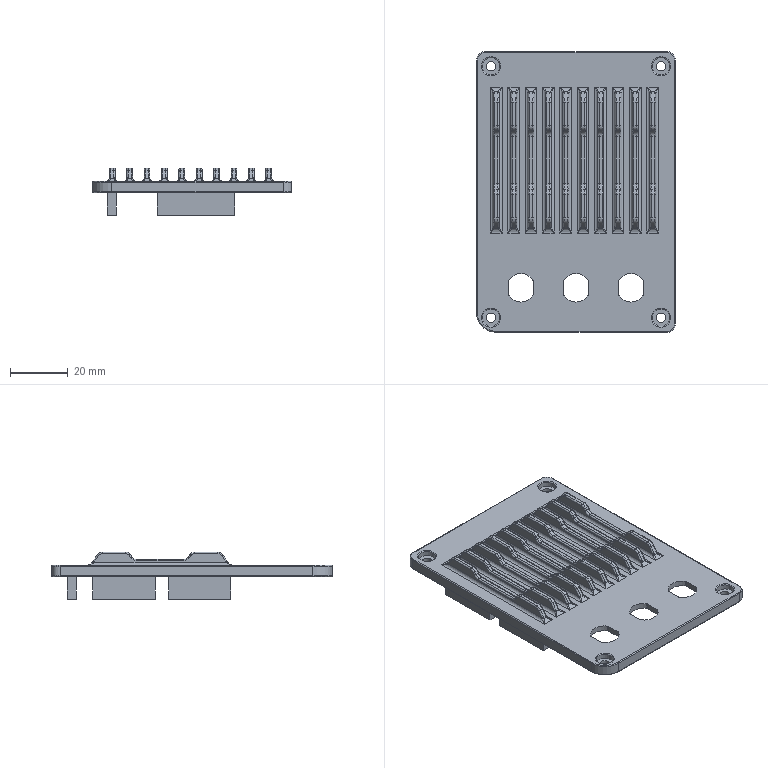NC program | NX | posted with a generic post | part box 68.665 x 96.782 x 16.5 mm
Lines 1 to 838 of 111885:
N10 G17 G21 G94 G90
(ADAPTIVE_MILLING , TOOL : D8平刀)
N12 T01 M6
N14 G53
N16 G17 G0 G90 X-18.024 Y-47.035 S5500 M3
N18 G43 Z20. H1
N20 Z-15.
N22 G94 G1 X-18.035 Y-46.886 Z-15.937 F2500.
N24 X-18.047 Y-46.736 Z-16.308
N26 X-18.058 Y-46.587 Z-16.58
N28 X-18.07 Y-46.437 Z-16.8
N30 X-18.081 Y-46.287 Z-16.984
N32 X-18.093 Y-46.138 Z-17.142
N34 X-18.104 Y-45.988 Z-17.28
N36 X-18.116 Y-45.839 Z-17.4
N38 X-18.127 Y-45.689 Z-17.505
N40 X-18.139 Y-45.54 Z-17.598
N42 X-18.15 Y-45.39 Z-17.679
N44 X-18.162 Y-45.241 Z-17.75
N46 X-18.173 Y-45.091 Z-17.81
N48 X-18.185 Y-44.941 Z-17.862
N50 X-18.196 Y-44.792 Z-17.905
N52 X-18.208 Y-44.642 Z-17.939
N54 X-18.219 Y-44.493 Z-17.966
N56 X-18.231 Y-44.343 Z-17.985
N58 X-18.242 Y-44.194 Z-17.996
N60 X-18.254 Y-44.044 Z-18.
N62 X-18.357 Y-42.702
N64 G3 X-18.789 Y-42.048 R0.809
N66 X-21.386 Y-41.32 R7.175
N68 X-27.459 Y-41.027 R57.317
N70 G1 X-36.427 Y-40.999
N72 X-55.027 Y-40.998
N74 G2 X-57.966 Y-39.532 R4.191
N76 X-59.796 Y-35.801 R8.355
N78 X-60.407 Y-30.293 R28.097
N80 X-60.498 Y-18.219 R430.715
N82 G1 Y35.526
N84 G2 X-58.974 Y38.514 R4.209
N86 X-55.153 Y40.331 R8.57
N88 X-49.493 Y40.917 R29.989
N90 X-37.268 Y40.998 R500.475
N92 G1 X55.025
N94 G2 X58.012 Y39.474 R4.21
N96 X59.796 Y35.792 R8.462
N98 X60.407 Y30.284 R28.108
N100 X60.498 Y17.76 R443.096
N102 G1 X60.496 Y-35.574
N104 G2 X58.937 Y-38.546 R4.252
N106 X55.241 Y-40.309 R8.541
N108 X49.808 Y-40.906 R28.315
N110 X37.284 Y-40.998 R440.918
N112 G1 X-15.616 Y-40.997
N114 G2 X-19.503 Y-40.574 R35.862
N116 G3 X-28.295 Y-40.042 R73.532
N118 X-40.552 Y-39.999 R802.999
N120 G1 X-52.652 Y-39.986
N122 G2 X-56.995 Y-37.488 R5.92
N124 X-58.825 Y-33.088 R11.007
N126 X-59.417 Y-26.824 R36.92
N128 X-59.498 Y-14.824 R522.113
N130 G1 X-59.494 Y32.976
N132 G2 X-57.007 Y37.48 R5.89
N134 X-52.54 Y39.333 R11.041
N136 X-46.275 Y39.917 R37.132
N138 X-32.626 Y39.998 R634.54
N140 G1 X52.473 Y39.994
N142 G2 X56.977 Y37.507 R5.892
N144 X58.832 Y33.041 R11.036
N146 X59.42 Y26.701 R37.884
N148 X59.498 Y14.252 R560.033
N150 G1 X59.494 Y-32.973
N152 G2 X57.005 Y-37.48 R5.892
N154 X52.538 Y-39.333 R11.051
N156 X46.348 Y-39.914 R36.953
N158 X32.549 Y-39.998 R617.93
N160 G1 X-13.551 Y-39.996
N162 G2 X-19.327 Y-39.564 R60.425
N164 G3 X-31.649 Y-39.023 R126.66
N166 G1 X-42.727 Y-39.
N168 G2 X-50.603 Y-38.979 R361.013
N170 X-56.053 Y-35.713 R6.95
N172 X-57.853 Y-30.884 R12.982
N174 X-58.422 Y-24.165 R43.91
N176 X-58.497 Y-11.341 R622.794
N178 G1 Y30.501
N180 G2 X-55.258 Y36.52 R6.96
N182 X-50.371 Y38.355 R12.933
N184 X-43.801 Y38.914 R42.861
N186 X-29.552 Y38.997 R688.41
N188 G1 X50.024 Y38.996
N190 G2 X56.078 Y35.67 R6.975
N192 X57.845 Y30.91 R13.
N194 X58.417 Y24.342 R43.075
N196 X58.497 Y11.592 R588.723
N198 G1 Y-30.508
N200 G2 X55.255 Y-36.524 R6.96
N202 X50.365 Y-38.354 R12.95
N204 X43.795 Y-38.914 R42.956
N206 X29.546 Y-38.997 R687.558
N208 G1 X-41.926 Y-38.99
N210 X-42.824 Y-38.651
N212 X-43.318 Y-38.533
N214 X-45.542
N216 G2 X-49.791 Y-38.012 R65.446
N218 X-55.19 Y-34.009 R8.027
N220 X-56.901 Y-28.83 R15.162
N222 X-57.434 Y-21.581 R53.165
N224 X-57.497 Y-9.206 R747.389
N226 G1 X-57.496 Y28.401
N228 G2 X-56.558 Y32.598 R8.417
N230 X-52.522 Y36.174 R8.634
N232 X-49.759 Y37.123 R16.528
N234 G1 X-49.065 Y37.589
N236 X-47.951 Y38.108
N238 X-46.764 Y38.426
N240 X-45.541 Y38.533
N242 X41.742
N244 G2 X44.4 Y38.26 R25.807
N246 G3 X48.887 Y38.011 R110.178
N248 G2 X55.038 Y34.214 R7.74
N250 X56.827 Y29.214 R14.237
N252 X57.418 Y22.196 R46.869
N254 X57.497 Y9.371 R617.595
N256 G1 X57.495 Y-28.549
N258 G2 X56.249 Y-33.109 R8.041
N260 X52.044 Y-36.384 R9.12
N262 X49.762 Y-37.12 R20.578
N264 G1 X49.065 Y-37.589
N266 X47.951 Y-38.108
N268 X46.764 Y-38.426
N270 X45.541 Y-38.533
N272 X-45.542
N274 X-46.767 Y-38.425
N276 X-47.954 Y-38.107
N278 G2 X-51.432 Y-36.143 R16.867
N280 X-55.071 Y-30.79 R11.246
N282 X-56.224 Y-24.461 R25.855
N284 X-56.487 Y-14.717 R142.012
N286 G1 X-56.496 Y-7.442
N288 Y26.451
N290 G2 X-55.941 Y30.289 R10.786
N292 X-52.207 Y34.579 R8.433
N294 G3 X-51.646 Y35.009 R1.591
N296 G1 X-50.941 Y36.015
N298 X-50.072 Y36.884
N300 X-49.642 Y37.185
N302 X-50.072 Y36.884
N304 X-50.941 Y36.015
N306 G2 X-51.941 Y34.587 R25.439
N308 G3 X-54.042 Y32.077 R20.332
N310 X-55.608 Y27.427 R10.728
N312 X-55.881 Y21.436 R54.834
N314 G1 X-55.896 Y15.061
N316 X-55.895 Y-10.764
N318 G3 X-55.717 Y-22.611 R250.597
N320 X-54.839 Y-29.065 R32.206
N322 X-51.872 Y-34.56 R12.101
N324 G1 X-51.647 Y-35.006
N326 X-50.943 Y-36.013
N328 X-50.074 Y-36.882
N330 X-49.067 Y-37.587
N332 X-50.074 Y-36.882
N334 X-50.943 Y-36.013
N336 X-51.647 Y-35.006
N338 X-52.166 Y-33.893
N340 G3 X-53.061 Y-31.219 R40.034
N342 G2 X-54.628 Y-22.76 R33.252
N344 X-54.886 Y-12.715 R158.699
N346 G1 X-54.896 Y-5.515
N348 X-54.895 Y16.635
N350 G2 X-54.749 Y25.032 R140.526
N352 X-53.73 Y29.696 R13.542
N354 X-52.612 Y31.732 R19.33
N356 G3 X-52.484 Y32.708 R4.161
N358 G1 X-52.165 Y33.895
N360 X-51.658 Y34.982
N362 X-52.165 Y33.895
N364 X-52.484 Y32.708
N366 G2 X-52.835 Y30.75 R6.595
N368 G3 X-54.178 Y23.101 R26.201
N370 X-54.295 Y12.153 R275.058
N372 G1 X-54.294 Y-8.797
N374 G3 X-54.102 Y-21.169 R254.458
N376 X-52.866 Y-29.538 R38.244
N378 G1 X-52.591 Y-30.55
N380 G3 X-52.484 Y-32.705 R13.839
N382 G1 X-52.271 Y-33.502
N384 X-52.484 Y-32.705
N386 G2 X-52.591 Y-30.55 R13.839
N388 G3 X-52.626 Y-27.217 R50.842
N390 G2 X-53.277 Y-12.198 R158.848
N392 G1 X-53.295 Y-2.448
N394 X-53.287 Y27.951
N396 G2 X-52.898 Y28.734 R3.274
N398 G3 X-52.591 Y29.483 R2.198
N400 G2 X-52.558 Y31.857 R26.948
N402 G3 X-52.591 Y29.333 R29.24
N404 X-52.694 Y19.519 R257.099
N406 G1 X-52.695 Y-24.756
N408 X-52.591 Y-25.224
N410 Y-27.849
N412 Y29.376
N414 G3 X-52.954 Y30.046 R0.801
N416 G1 X-53.233 Y30.227
N418 X-54.544 Y31.082 Z-17.9
N420 G2 X-54.911 Y31.373 R1.372 F15000.
N422 X-55.08 Y31.865 R0.808
N424 G1 X-55.071 Y32.596
N426 G2 X-54.931 Y33.308 R3.318
N428 G1 X-54.719 Y33.972
N430 X-54.496 Y34.631
N432 G2 X-53.279 Y36.79 R8.173
N434 G1 X-52.849 Y37.337
N436 X-52.412 Y37.878
N438 G2 X-49.82 Y39.92 R8.545
N440 X-47.867 Y40.563 R7.242
N442 X-44.961 Y40.828 R17.468
N444 G1 X41.746 Y41.423
N446 G2 X42.536 Y40.78 R0.8
N448 G1 X42.602 Y40.45
N450 X42.913 Y38.916 Z-18. F2500.
N452 G3 X43.506 Y38.374 R0.801
N454 G2 X45.905 Y37.69 R11.19
N456 G1 X48.563 Y37.089
N458 G2 X54.347 Y32.308 R8.991
N460 X55.971 Y26.713 R17.615
N462 X56.449 Y18.858 R66.245
N464 X56.497 Y7.383 R752.762
N466 G1 X56.496 Y-26.467
N468 G2 X55.934 Y-30.304 R10.723
N470 X52.176 Y-34.594 R8.431
N472 G3 X51.646 Y-35.009 R1.478
N474 G1 X50.941 Y-36.015
N476 X50.072 Y-36.884
N478 X49.642 Y-37.185
N480 X50.072 Y-36.884
N482 X50.941 Y-36.015
N484 G2 X51.942 Y-34.585 R25.841
N486 G3 X53.935 Y-32.237 R22.088
N488 X55.603 Y-27.471 R10.602
N490 X55.88 Y-21.63 R52.787
N492 G1 X55.896 Y-15.18
N494 X55.895 Y10.795
N496 G3 X55.71 Y22.642 R240.339
N498 X54.806 Y29.016 R30.462
N500 X52.302 Y33.745 R11.117
N502 X48.519 Y36.143 R9.866
N504 G1 X47.608 Y36.81
N506 X46.249 Y37.552
N508 X45.757 Y37.735
N510 X46.249 Y37.552
N512 X47.608 Y36.81
N514 X48.847 Y35.882
N516 G2 X51.722 Y32.612 R21.631
N518 X54.12 Y26.42 R16.459
N520 X54.795 Y19.033 R48.127
N522 X54.896 Y5.384 R526.187
N524 G1 X54.895 Y-17.216
N526 G2 X54.734 Y-25.238 R120.855
N528 X53.576 Y-30.022 R12.875
N530 X52.617 Y-31.72 R25.473
N532 G3 X52.484 Y-32.708 R3.891
N534 G1 X52.165 Y-33.895
N536 X51.658 Y-34.982
N538 X52.165 Y-33.895
N540 X52.484 Y-32.708
N542 G2 X52.9 Y-30.542 R6.783
N544 G3 X54.178 Y-23.096 R26.081
N546 X54.296 Y-12.147 R274.789
N548 G1 X54.294 Y8.653
N550 G3 X54.118 Y20.5 R256.148
N552 X53.211 Y27.328 R34.49
N554 X52.338 Y29.883 R19.16
N556 G1 X52.152 Y30.738
N558 X51.611 Y32.189
N560 X50.869 Y33.548
N562 X49.942 Y34.787
N564 X50.869 Y33.548
N566 X51.611 Y32.189
N568 X52.152 Y30.738
N570 X52.481 Y29.226
N572 G2 X52.658 Y26.199 R227.716
N574 X53.279 Y11.759 R149.003
N576 G1 X53.295 Y2.159
N578 X53.287 Y-27.549
N580 G2 X52.882 Y-28.426 R5.062
N582 G3 X52.591 Y-29.196 R2.618
N584 G2 X52.558 Y-31.857 R31.387
N586 G3 X52.591 Y-29.196 R31.387
N588 X52.695 Y-17.191 R349.902
N590 G1 X52.687 Y23.202
N592 X52.591 Y23.618
N594 Y27.218
N596 Y-29.032
N598 G3 X53.506 Y-29.833 R0.808
N600 G1 X54.547 Y-29.694
N602 X54.696 Y-29.674 Z-17.996
N604 X54.844 Y-29.654 Z-17.985
N606 X54.993 Y-29.634 Z-17.966
N608 X55.142 Y-29.614 Z-17.939
N610 X55.29 Y-29.595 Z-17.905
N612 X55.439 Y-29.575 Z-17.862
N614 X55.588 Y-29.555 Z-17.81
N616 X55.736 Y-29.535 Z-17.75
N618 X55.885 Y-29.515 Z-17.679
N620 X56.034 Y-29.495 Z-17.598
N622 X56.182 Y-29.475 Z-17.505
N624 X56.331 Y-29.456 Z-17.4
N626 X56.48 Y-29.436 Z-17.28
N628 X56.628 Y-29.416 Z-17.142
N630 X56.777 Y-29.396 Z-16.984
N632 X56.926 Y-29.376 Z-16.8
N634 X57.074 Y-29.356 Z-16.58
N636 X57.223 Y-29.336 Z-16.308
N638 X57.372 Y-29.317 Z-15.937
N640 X57.521 Y-29.297 Z-15.
N642 G0 Z20.
N644 X13.922 Y-4.732
N646 Z3.
N648 G3 X13.922 Y-4.732 Z2.605 I3.157 J1.73
N650 X13.922 Y-4.732 Z2.21 I3.157 J1.73
N652 X13.922 Y-4.732 Z1.816 I3.157 J1.73
N654 X13.922 Y-4.732 Z1.421 I3.157 J1.73
N656 X13.922 Y-4.732 Z1.026 I3.157 J1.73
N658 X13.922 Y-4.732 Z0.631 I3.157 J1.73
N660 X13.922 Y-4.732 Z0.236 I3.157 J1.73
N662 X13.922 Y-4.732 Z-0.159 I3.157 J1.73
N664 X13.922 Y-4.732 Z-0.553 I3.157 J1.73
N666 X13.922 Y-4.732 Z-0.948 I3.157 J1.73
N668 X13.922 Y-4.732 Z-1.343 I3.157 J1.73
N670 X13.922 Y-4.732 Z-1.738 I3.157 J1.73
N672 X13.922 Y-4.732 Z-2.133 I3.157 J1.73
N674 X13.922 Y-4.732 Z-2.528 I3.157 J1.73
N676 X13.922 Y-4.732 Z-2.922 I3.157 J1.73
N678 X13.922 Y-4.732 Z-3.317 I3.157 J1.73
N680 X13.922 Y-4.732 Z-3.712 I3.157 J1.73
N682 X13.922 Y-4.732 Z-4.107 I3.157 J1.73
N684 X13.922 Y-4.732 Z-4.502 I3.157 J1.73
N686 X13.922 Y-4.732 Z-4.896 I3.157 J1.73
N688 X13.922 Y-4.732 Z-5.291 I3.157 J1.73
N690 X13.922 Y-4.732 Z-5.686 I3.157 J1.73
N692 X13.922 Y-4.732 Z-6.081 I3.157 J1.73
N694 X13.922 Y-4.732 Z-6.476 I3.157 J1.73
N696 X13.922 Y-4.732 Z-6.871 I3.157 J1.73
N698 X13.922 Y-4.732 Z-7.265 I3.157 J1.73
N700 X13.922 Y-4.732 Z-7.66 I3.157 J1.73
N702 X13.922 Y-4.732 Z-8.055 I3.157 J1.73
N704 X13.922 Y-4.732 Z-8.45 I3.157 J1.73
N706 X13.922 Y-4.732 Z-8.845 I3.157 J1.73
N708 X13.922 Y-4.732 Z-9.24 I3.157 J1.73
N710 X13.922 Y-4.732 Z-9.634 I3.157 J1.73
N712 X17.08 Y0.598 Z-9.899 R-3.6
N714 X20.582 Y-4.008 R-3.622
N716 X19.288 Y-0.074 R3.686
N718 X12.982 Y-2.744 R3.8
N720 X20.455 Y-0.577 R-4.131
N722 X12.462 Y-3.394 R4.367
N724 X21.31 Y-0.982 R-4.66
N726 X11.954 Y-3.812 R4.929
N728 X22.125 Y-1.568 R-5.217
N730 X11.355 Y-3.699 R5.503
N732 X17.809 Y-8.754 R5.797
N734 X22.866 Y-2.311 R5.797
N736 X10.718 Y-3.256 R6.096
N738 X23.495 Y-3.461 R6.398
N740 X10.116 Y-2.46 R6.708
N742 X23.763 Y-5.269 R7.018
N744 X10.587 Y0.902 R7.325
N746 X17.282 Y-10.684 R7.598
N748 X23.733 Y1.042 R7.765
N750 X8.775 Y-3.24 R8.034
N752 X25.07 Y-5.539 R8.344
N754 X11.862 Y4.14 R8.646
N756 X13.05 Y-11.085 R8.881
N758 X25.345 Y0.901 R9.102
N760 X7.416 Y-2.438 R9.403
N762 X23.796 Y-10.079 R9.707
N764 X22.117 Y5.596 R9.937
N766 X7.112 Y-6.057 R10.164
N768 X27.209 Y-5.802 R10.473
N770 X11.138 Y6.206 R10.773
N772 X11.116 Y-12.45 R10.996
N774 X27.557 Y1.242 R11.252
N776 X5.69 Y0.218 R11.571
N778 X19.657 Y-14.657 R11.858
N780 X26.065 Y5.115 R12.067
N782 X4.644 Y-0.954 R12.341
N784 X22.622 Y-14.425 R12.634
N786 X25.056 Y7.141 R12.85
N788 X3.701 Y-3.375 R13.119
N790 X26.346 Y-12.784 R13.419
N792 X24.449 Y8.542 R13.647
N794 X3.398 Y-6.719 R13.908
N796 X30.019 Y-9.032 R14.232
N798 X11.548 Y10.621 R14.525
N800 X8.296 Y-15.141 R14.778
N802 X31.888 Y0.068 R15.07
N804 X4.861 Y6.714 R15.386
N806 X9.873 Y-17.037 R15.615
N808 X32.549 Y0.787 R15.877
N810 X3.137 Y5.689 R16.195
N812 X9.362 Y-17.671 R16.421
N814 X33.375 Y0.786 R16.681
N816 X3.114 Y7.069 R16.993
N818 X9.8 Y-18.782 R17.219
N820 X34.348 Y0.044 R17.486
N822 X3.358 Y8.66 R17.794
N824 X7.554 Y-18.495 R18.014
N826 X35.315 Y-0.998 R18.294
N828 X4.957 Y11.349 R18.594
N830 X6.715 Y-18.932 R18.823
N832 X35.84 Y1.01 R19.121
N834 X1.951 Y9.53 R19.435
N836 X8.647 Y-20.947 R19.66
N838 X35.751 Y4.276 R19.96
N840 X-2.13 Y4.25 R20.294
N842 X12.106 Y-23.058 R20.524
N844 X35.471 Y6.921 R20.808
N846 X-4.227 Y-0.917 R21.155
N848 X15.775 Y-24.466 R21.396
N850 X32.689 Y12.192 R21.664
N852 X-5.076 Y-5.325 R22.029
N854 X26.972 Y-23.076 R22.328
N856 X22.925 Y18.949 R22.561
N858 X-1.834 Y-16.352 R22.9
N860 X38.208 Y-12.816 R23.25
N862 X17.957 Y20.595 R23.473
N864 X1.401 Y-21.184 R23.772
N866 X41.223 Y-0.98 R24.144
N868 X11.686 Y20.92 R24.409
N870 X4.74 Y-24.587 R24.647
N872 X41.909 Y0.666 R25.01
N874 X31.653 Y17.584 R25.134
N876 X14.857 Y22.253 R25.177
N878 G1 X14.343 Y22.073
N880 G3 X10.085 Y21.391 R27.002
N882 X-8.581 Y-2.536 R25.356
N884 X12.199 Y-28.283 R25.617
N886 G1 X21.125 Y-28.272
N888 G3 X28.926 Y-25.929 R21.19
N890 X42.341 Y-8.736 R25.853
N892 X42.324 Y2.009 R732.069
N894 X40.442 Y8.427 R19.199
N896 X16.607 Y23.211 R26.063
N898 X16.027 Y22.884 R0.976
N900 G1 X15.231 Y22.384
N902 X14.343 Y22.073
N904 X13.408 Y21.968
N906 G3 X10.069 Y21.942 R56.93
N908 X4.901 Y20.303 R15.834
N910 X-9.186 Y0.684 R26.1
N912 X8.747 Y-28.275 R26.437
N914 G1 X12.27 Y-28.283
N916 X8.277 Y-28.273
N918 G2 X4.798 Y-27.153 R11.032
N920 X-8.627 Y-11.616 R26.571
N922 X3.238 Y20.003 R26.838
N924 X7.81 Y21.965 R19.277
N926 G1 X10.461 Y21.968
N928 X6.555 Y21.954
N930 G3 X2.769 Y20.637 R10.92
N932 X-6.032 Y12.539 R25.401
N934 X2.67 Y-27.009 R27.771
N936 X5.23 Y-28.26 R18.595
N938 G1 X5.378 Y-28.283
N940 X8.453
N942 X4.967 Y-28.268
N944 G2 X2.055 Y-27.162 R8.703
N946 X-6.045 Y-19.737 R25.808
N948 X-1.162 Y18.624 R28.271
N950 X4.469 Y21.917 R19.041
N952 G1 X4.698 Y21.968
N954 X6.723
N956 X3.717 Y21.954
N958 G3 X0.336 Y20.65 R9.047
N960 X-6.449 Y14.378 R24.127
N962 X-1.369 Y-25.916 R29.166
N964 X2.379 Y-28.246 R17.939
N966 G1 X2.572 Y-28.283
N968 X5.197
N970 G2 X2.171 Y-28.261 R46.951
N972 X-0.595 Y-27.033 R8.055
N974 X-7.246 Y-20.497 R25.412
N976 X-4.356 Y17.596 R29.667
N978 X0.933 Y21.521 R20.08
N980 X2.104 Y21.968 R4.738
N982 G1 X3.904
N984 X1.281 Y21.955
N986 G3 X-1.607 Y20.831 R7.604
N988 X-6.893 Y16.09 R21.347
N990 X-4.37 Y-25.159 R30.537
N992 X-0.136 Y-28.226 R17.588
N994 G1 X0.113 Y-28.283
N996 X2.363
N998 G2 X-0.208 Y-28.265 R68.809
N1000 X-2.728 Y-27.092 R6.893
N1002 X-8.174 Y-21.639 R23.635
N1004 X-7.059 Y16.71 R31.067
N1006 X-1.968 Y21.177 R20.855
N1008 X-0.248 Y21.965 R6.683
N1010 G1 X1.435 Y21.968
N1012 X-0.961 Y21.955
N1014 G3 X-3.872 Y20.727 R7.198
N1016 X-8.772 Y15.971 R20.851
N1018 X-6.968 Y-24.509 R31.896
N1020 X-2.659 Y-28.083 R18.038
N1022 X-2.133 Y-28.283 R1.48
N1024 G1 X-0.033
N1026 G2 X-2.461 Y-28.26 R30.8
N1028 X-4.864 Y-27.059 R6.532
N1030 X-9.719 Y-21.933 R22.632
N1032 X-9.441 Y15.962 R32.44
N1034 X-4.492 Y20.889 R21.458
N1036 X-2.476 Y21.949 R9.122
N1038 X-0.776 Y21.968 R22.711
N1040 G1 X-3.09 Y21.953
N1042 G3 X-5.893 Y20.7 R6.909
N1044 X-10.505 Y15.982 R20.109
N1046 X-15.883 Y-9.95 R33.041
N1048 X-8.624 Y-24.749 R32.456
N1050 X-4.712 Y-28.104 R16.316
N1052 X-4.217 Y-28.283 R1.28
N1054 G1 X-2.267
N1056 X-4.442 Y-28.279
N1058 G2 X-6.653 Y-27.206 R5.519
N1060 X-10.892 Y-22.732 R20.246
N1062 X-11.533 Y15.438 R33.758
N1064 X-6.721 Y20.694 R21.748
N1066 X-4.463 Y21.956 R7.941
N1068 G1 X-2.881 Y21.968
N1070 X-5.055 Y21.953
N1072 G3 X-7.671 Y20.787 R6.398
N1074 X-12.009 Y16.275 R18.854
N1076 X-17.976 Y-1.343 R33.656
N1078 X-11.261 Y-23.741 R34.427
N1080 X-7.241 Y-27.766 R18.41
N1082 X-6.303 Y-28.272 R2.986
N1084 G1 X-4.35 Y-28.283
N1086 G2 X-6.543 Y-28.259 R23.675
N1088 X-8.835 Y-27. R5.969
N1090 X-13.046 Y-22.101 R21.147
N1092 X-13.682 Y14.694 R35.11
N1094 X-8.987 Y20.38 R22.673
N1096 X-6.463 Y21.939 R9.342
N1098 G1 X-6.303 Y21.968
N1100 X-4.878
N1102 G3 X-6.976 Y21.951 R153.906
N1104 X-9.6 Y20.72 R6.251
N1106 X-13.784 Y16.15 R18.554
N1108 X-19.27 Y0.666 R34.372
N1110 X-13.344 Y-23.268 R35.794
N1112 X-9.444 Y-27.544 R19.103
N1114 X-8.306 Y-28.252 R5.009
N1116 G1 X-8.139 Y-28.283
N1118 X-6.339
N1120 X-8.289
N1122 G2 X-10.183 Y-27.388 R4.394
N1124 X-13.792 Y-23.516 R16.863
N1126 X-19.684 Y-8.078 R35.238
N1128 X-15.269 Y14.79 R36.058
N1130 X-10.806 Y20.367 R22.036
N1132 X-8.336 Y21.936 R9.044
N1134 G1 X-8.073 Y21.968
N1136 X-6.798
N1138 G2 X-8.634 Y21.994 R75.24
N1140 G3 X-11.034 Y20.973 R5.349
N1142 X-14.893 Y16.962 R16.306
N1144 X-19.949 Y5.357 R33.327
N1146 X-15.55 Y-22.488 R37.277
N1148 X-11.582 Y-27.298 R20.326
N1150 X-10.182 Y-28.245 R6.083
N1152 G1 X-9.986 Y-28.283
N1154 X-8.261
N1156 X-10.211 Y-28.278
N1158 G2 X-12.165 Y-27.259 R4.788
N1160 X-15.708 Y-23.195 R17.372
N1162 X-21.156 Y-8.054 R36.295
N1164 X-17.19 Y14.258 R37.303
N1166 X-12.887 Y20.076 R22.943
N1168 X-9.834 Y22.067 R8.943
N1170 X-9.257 Y22.148 R1.232
N1172 G3 X-8.447 Y21.998 R3.368
N1174 G2 X-9.472 Y22.207 R4.203
N1176 G3 X-11.371 Y21.859 R3.289
N1178 X-14.86 Y19.128 R10.99
N1180 X-19.346 Y11.845 R26.804
N1182 X-17.455 Y-22.078 R38.528
N1184 X-13.658 Y-27.039 R21.19
N1186 X-12.036 Y-28.229 R8.142
N1188 G1 X-11.797 Y-28.283
N1190 X-10.072
N1192 X-11.947
N1194 G2 X-13.816 Y-27.351 R4.246
N1196 X-17.264 Y-23.372 R16.234
N1198 X-22.225 Y-10.633 R36.351
N1200 X-19.159 Y13.539 R38.744
N1202 X-14.834 Y19.881 R24.34
N1204 X-11.896 Y22.057 R10.371
N1206 G3 X-10.848 Y22.379 R7.877
N1208 G2 X-9.958 Y22.42 R1.402
N1210 G1 X-9.401 Y22.184
N1212 G3 X-10.391 Y22.512 R3.074
N1214 X-11.383 Y22.183 R2.915
N1216 G2 X-12.556 Y21.964 R6.52
N1218 G3 X-15.114 Y20.531 R6.356
N1220 X-18.983 Y15.715 R18.806
N1222 X-23.402 Y2.851 R36.452
N1224 X-19.24 Y-21.812 R39.66
N1226 X-15.465 Y-26.976 R21.212
N1228 X-13.811 Y-28.224 R8.055
N1230 G1 X-13.558 Y-28.283
N1232 X-11.908
N1234 X-13.783 Y-28.277
N1236 G2 X-15.783 Y-27.164 R4.757
N1238 X-19.207 Y-22.907 R17.283
N1240 X-23.97 Y-9.117 R37.764
N1242 X-20.812 Y13.392 R39.806
N1244 X-16.733 Y19.651 R24.375
N1246 X-13.764 Y21.922 R9.61
N1248 X-12.71 Y21.968 R4.266
N1250 G1 X-12.411 Y21.992
N1252 G2 X-13.994 Y21.968 R27.116
N1254 G3 X-16.26 Y20.943 R4.946
N1256 X-19.829 Y16.954 R15.407
N1258 X-24.066 Y6.941 R33.717
N1260 X-21.267 Y-21.018 R40.997
N1262 X-17.529 Y-26.622 R22.95
N1264 X-15.523 Y-28.232 R7.934
N1266 G1 X-15.294 Y-28.283
N1268 X-13.644
N1270 X-15.444
N1272 G2 X-17.188 Y-27.406 R3.956
N1274 X-20.351 Y-23.707 R14.743
N1276 X-24.713 Y-13.026 R35.805
N1278 X-22.859 Y12.306 R41.361
N1280 X-18.835 Y19.148 R26.098
N1282 X-15.697 Y21.785 R10.614
N1284 X-15.166 Y21.968 R1.645
N1286 G1 X-13.966
N1288 X-15.759 Y21.952
N1290 G3 X-18.195 Y20.724 R5.393
N1292 X-21.772 Y16.419 R16.343
N1294 X-25.815 Y5.928 R35.197
N1296 X-23.176 Y-20.359 R42.198
N1298 X-19.557 Y-26.239 R24.545
N1300 X-17.233 Y-28.229 R8.532
N1302 G1 X-16.994 Y-28.283
N1304 X-15.419
N1306 X-17.144
N1308 G2 X-18.839 Y-27.433 R3.883
N1310 X-21.924 Y-23.801 R14.208
N1312 X-26.081 Y-13.634 R35.483
N1314 X-24.65 Y11.707 R42.578
N1316 X-20.687 Y18.878 R26.934
N1318 X-17.511 Y21.7 R11.106
N1320 X-16.817 Y21.968 R1.94
N1322 G1 X-15.542
N1324 X-17.408 Y21.952
N1326 G3 X-19.818 Y20.741 R5.42
N1328 X-23.349 Y16.445 R16.1
N1330 X-27.223 Y6.36 R35.142
N1332 X-25.02 Y-19.757 R43.37
N1334 X-21.437 Y-25.972 R25.733
N1336 X-18.938 Y-28.22 R9.143
N1338 G1 X-18.669 Y-28.283
N1340 X-17.094
N1342 X-18.894 Y-28.277
N1344 G2 X-20.793 Y-27.197 R4.448
N1346 X-23.94 Y-23.136 R15.916
N1348 X-27.974 Y-11.932 R37.623
N1350 X-26.322 Y11.366 R43.619
N1352 X-22.535 Y18.579 R27.744
N1354 X-19.293 Y21.621 R11.561
N1356 X-18.46 Y21.968 R2.277
N1358 G1 X-17.26
N1360 X-19.05 Y21.952
N1362 G3 X-21.432 Y20.747 R5.316
N1364 X-24.843 Y16.593 R15.638
N1366 X-28.6 Y6.93 R34.697
N1368 X-26.761 Y-19.342 R44.505
N1370 X-23.172 Y-25.851 R26.36
N1372 X-20.649 Y-28.2 R9.599
N1374 G1 X-20.342 Y-28.283
N1376 X-18.767
N1378 X-20.492
N1380 G2 X-22.214 Y-27.385 R3.833
N1382 X-25.234 Y-23.667 R14.193
N1384 X-29.075 Y-13.817 R35.701
N1386 X-28.115 Y10.632 R44.886
N1388 X-24.326 Y18.319 R28.855
N1390 X-20.983 Y21.585 R11.95
N1392 X-20.099 Y21.968 R2.501
N1394 G1 X-18.899
N1396 X-20.685 Y21.952
N1398 G3 X-23.088 Y20.71 R5.343
N1400 X-26.518 Y16.423 R15.778
N1402 X-30.184 Y6.599 R35.222
N1404 X-28.456 Y-18.997 R45.606
N1406 X-25.015 Y-25.564 R27.318
N1408 X-22.295 Y-28.199 R9.883
N1410 G1 X-21.984 Y-28.283
N1412 X-20.484
N1414 X-22.134
N1416 G2 X-23.839 Y-27.392 R3.783
N1418 X-26.784 Y-23.751 R13.856
N1420 X-30.484 Y-14.282 R35.198
N1422 X-29.748 Y10.318 R45.976
N1424 X-26.108 Y18.041 R29.598
N1426 X-22.929 Y21.372 R12.748
N1428 X-21.805 Y21.955 R4.192
N1430 G1 X-20.518 Y21.968
N1432 G3 X-22.313 Y21.949 R36.92
N1434 X-24.678 Y20.718 R5.324
N1436 X-28.075 Y16.441 R15.583
N1438 X-31.659 Y6.751 R35.162
N1440 X-30.061 Y-18.866 R46.607
N1442 X-26.693 Y-25.471 R27.539
N1444 X-23.932 Y-28.195 R9.924
N1446 G1 X-23.612 Y-28.283
N1448 X-22.112
N1450 X-23.837 Y-28.277
N1452 G2 X-25.601 Y-27.276 R4.179
N1454 X-28.58 Y-23.395 R14.688
N1456 X-32.16 Y-13.614 R36.392
N1458 X-31.336 Y10.119 R46.954
N1460 X-27.727 Y17.98 R29.808
N1462 X-24.554 Y21.354 R12.759
N1464 X-23.387 Y21.959 R3.89
N1466 G1 X-22.112 Y21.968
N1468 G3 X-23.901 Y21.951 R93.217
N1470 X-26.367 Y20.63 R5.335
N1472 X-29.704 Y16.32 R15.78
N1474 X-33.195 Y6.624 R35.489
N1476 X-31.71 Y-18.592 R47.614
N1478 X-28.315 Y-25.44 R27.72
N1480 X-25.627 Y-28.156 R10.272
N1482 X-25.233 Y-28.283 R1.536
N1484 G1 X-23.733
N1486 X-25.383
N1488 G2 X-27.104 Y-27.364 R3.731
N1490 X-30.01 Y-23.663 R13.816
N1492 X-33.511 Y-14.356 R35.239
N1494 X-33.014 Y9.598 R48.016
N1496 X-29.468 Y17.718 R30.703
N1498 X-26.268 Y21.266 R13.224
N1500 X-24.965 Y21.961 R3.978
N1502 G1 X-23.698 Y21.968
N1504 X-25.483 Y21.952
N1506 G3 X-27.938 Y20.636 R5.296
N1508 X-31.246 Y16.343 R15.612
N1510 X-34.643 Y6.916 R35.387
N1512 X-35.691 Y-1.742 R48.114
N1514 X-35.66 Y-6.029 R80.735
N1516 X-32.837 Y-19.743 R46.655
N1518 X-29.511 Y-25.973 R24.679
N1520 X-27.153 Y-28.198 R9.014
N1522 G1 X-26.84 Y-28.283
N1524 X-25.34
N1526 X-27.065 Y-28.276
N1528 G2 X-28.877 Y-27.215 R4.258
N1530 X-31.793 Y-23.292 R14.718
N1532 X-35.198 Y-13.605 R36.6
N1534 X-35.691 Y-10.921 R101.572
N1536 G1 Y-5.446
N1538 G3 X-35.674 Y-14.248 R482.909
N1540 X-34.018 Y-20.621 R23.422
N1542 X-30.811 Y-26.329 R21.708
N1544 X-28.754 Y-28.198 R8.429
N1546 G1 X-28.44 Y-28.283
N1548 X-26.94
N1550 X-28.59
N1552 G2 X-30.282 Y-27.374 R3.672
N1554 X-33.14 Y-23.679 R13.389
N1556 X-35.899 Y-16.185 R26.364
N1558 X-35.796 Y-15.667 R1.292
N1560 G3 X-35.691 Y-13.983 R8.39
N1562 G2 X-35.796 Y-15.667 R8.39
N1564 G3 X-36.042 Y-17.981 R4.216
N1566 X-34.055 Y-23.773 R17.265
N1568 X-31.077 Y-27.668 R13.3
N1570 X-30.136 Y-28.265 R2.641
N1572 X-28.52 Y-28.283 R40.276
N1574 G1 X-30.17
N1576 G2 X-31.844 Y-27.383 R3.596
N1578 X-34.728 Y-23.526 R12.821
N1580 X-36.466 Y-18.187 R15.531
N1582 X-36.432 Y-17.091 R2.573
N1584 G3 X-35.983 Y-16.2 R3.443
N1586 G2 X-36.401 Y-17.022 R2.268
N1588 G3 X-36.846 Y-18.637 R2.822
N1590 X-35.997 Y-22.649 R10.405
N1592 X-32.839 Y-27.483 R13.353
N1594 X-31.757 Y-28.249 R3.645
N1596 G1 X-31.58 Y-28.283
N1598 X-30.155
N1600 X-31.73
N1602 G2 X-33.316 Y-27.438 R3.445
N1604 X-35.151 Y-25.294 R9.842
N1606 G3 X-35.744 Y-24.222 R7.969
N1608 G2 X-37.248 Y-19.205 R11.262
N1610 X-37.076 Y-17.883 R3.529
N1612 X-36.607 Y-17.351 R2.294
N1614 G1 X-36.528 Y-17.224
N1616 G2 X-37.164 Y-17.908 R4.081
N1618 G3 X-37.696 Y-19.772 R3.274
N1620 X-37.286 Y-22.398 R6.709
N1622 X-36.111 Y-23.708 R22.7
N1624 G1 X-35.454 Y-24.712
N1626 G3 X-37.247 Y-22.504 R9.112
N1628 G2 X-38.006 Y-20.367 R3.881
N1630 X-37.734 Y-18.417 R3.89
N1632 X-37.272 Y-18.016 R1.239
N1634 G1 X-37.113 Y-17.857
N1636 G2 X-37.687 Y-18.276 R2.294
N1638 G3 X-38.427 Y-19.86 R2.398
N1640 X-38.242 Y-21.626 R3.451
N1642 G1 X-38.075 Y-21.839
N1644 X-37.198 Y-22.544
N1646 X-38.192 Y-21.745
N1648 G2 X-38.674 Y-19.875 R2.53
N1650 X-38.247 Y-18.652 R2.108
N1652 G1 X-38.069 Y-18.516
N1654 G2 X-37.297 Y-18.618 R0.882
N1656 X-36.903 Y-19.355 Z-9.844 R0.911
N1658 G1 X-36.846 Y-20.048 Z-9.799
N1660 X-36.823 Y-20.327 F15000.
N1662 X-36.789 Y-20.719 Z-9.824 F2500.
N1664 X-36.769 Y-21.112 Z-9.849
N1666 G2 X-37.135 Y-21.77 Z-9.899 R0.892
N1668 X-38.192 Y-21.745 R0.88
N1670 X-38.875 Y-20.432 R1.873
N1672 X-38.603 Y-18.858 R2.352
N1674 X-38.069 Y-18.516 R1.024